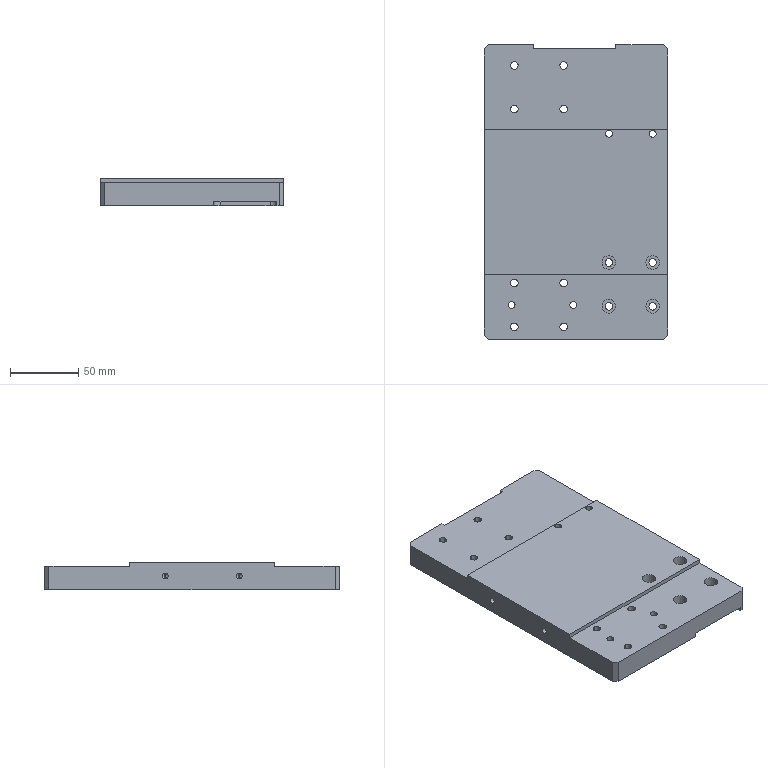Part | SolidWorks | features HoleWzd 8, ICE 2, Chamfer 1, Extrusion 1 | 1 solid | 116 faces | box 134 x 215 x 20 mm | volume 503550 mm3 | cylinder 70 | plane 34 | cone 12 | commonest cylinder face diameters 10 x26 5.5 x24 5 x12 4.2 x8